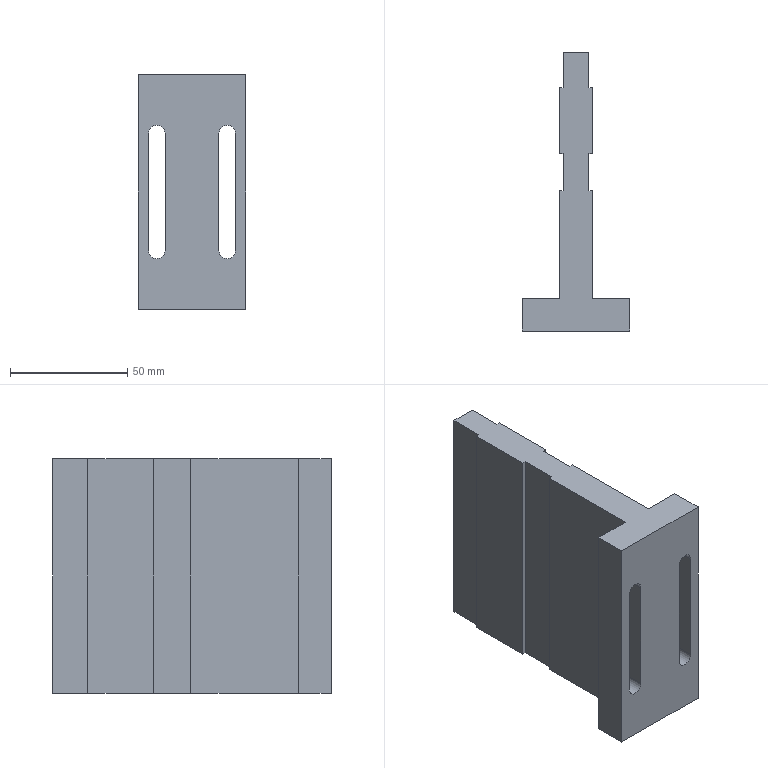Part | SolidWorks | features ICE 2, MirrorPattern 2, Extrusion 1 | 1 solid | 30 faces | box 46 x 119 x 100 mm | volume 191222 mm3 | plane 26 | cylinder 4 | commonest cylinder face diameters 7 x4
STEP:
#1=CARTESIAN_POINT('',(-5.5,119.,-50.));
#2=VERTEX_POINT('',#1);
#3=CARTESIAN_POINT('',(-5.5,119.,50.));
#4=VERTEX_POINT('',#3);
#5=CARTESIAN_POINT('',(-5.5,119.,50.));
#6=DIRECTION('',(0.,0.,1.));
#7=VECTOR('',#6,1000.);
#8=LINE('',#5,#7);
#9=EDGE_CURVE('',#2,#4,#8,.T.);
#10=ORIENTED_EDGE('',*,*,#9,.T.);
#11=CARTESIAN_POINT('',(5.5,119.,50.));
#12=VERTEX_POINT('',#11);
#13=CARTESIAN_POINT('',(7.,119.,50.));
#14=DIRECTION('',(-1.,0.,0.));
#15=VECTOR('',#14,1000.);
#16=LINE('',#13,#15);
#17=EDGE_CURVE('',#12,#4,#16,.T.);
#18=ORIENTED_EDGE('',*,*,#17,.F.);
#19=CARTESIAN_POINT('',(5.5,119.,-50.));
#20=VERTEX_POINT('',#19);
#21=CARTESIAN_POINT('',(5.5,119.,50.));
#22=DIRECTION('',(0.,0.,1.));
#23=VECTOR('',#22,1000.);
#24=LINE('',#21,#23);
#25=EDGE_CURVE('',#20,#12,#24,.T.);
#26=ORIENTED_EDGE('',*,*,#25,.F.);
#27=CARTESIAN_POINT('',(7.,119.,-50.));
#28=DIRECTION('',(-1.,0.,0.));
#29=VECTOR('',#28,1000.);
#30=LINE('',#27,#29);
#31=EDGE_CURVE('',#20,#2,#30,.T.);
#32=ORIENTED_EDGE('',*,*,#31,.T.);
#33=EDGE_LOOP('',(#10,#18,#26,#32));
#34=FACE_OUTER_BOUND('',#33,.T.);
#35=CARTESIAN_POINT('',(7.,119.,50.));
#36=DIRECTION('',(0.,-1.,0.));
#37=DIRECTION('',(0.,0.,-1.));
#38=AXIS2_PLACEMENT_3D('',#35,#36,#37);
#39=PLANE('',#38);
#40=ADVANCED_FACE('',(#34),#39,.F.);
#41=CARTESIAN_POINT('',(-7.,104.,50.));
#42=VERTEX_POINT('',#41);
#43=CARTESIAN_POINT('',(-7.,104.,-50.));
#44=VERTEX_POINT('',#43);
#45=CARTESIAN_POINT('',(-7.,104.,50.));
#46=DIRECTION('',(0.,0.,-1.));
#47=VECTOR('',#46,1000.);
#48=LINE('',#45,#47);
#49=EDGE_CURVE('',#42,#44,#48,.T.);
#50=ORIENTED_EDGE('',*,*,#49,.T.);
#51=CARTESIAN_POINT('',(-7.,76.,-50.));
#52=VERTEX_POINT('',#51);
#53=CARTESIAN_POINT('',(-7.,119.,-50.));
#54=DIRECTION('',(0.,-1.,0.));
#55=VECTOR('',#54,1000.);
#56=LINE('',#53,#55);
#57=EDGE_CURVE('',#44,#52,#56,.T.);
#58=ORIENTED_EDGE('',*,*,#57,.T.);
#59=CARTESIAN_POINT('',(-7.,76.,50.));
#60=VERTEX_POINT('',#59);
#61=CARTESIAN_POINT('',(-7.,76.,50.));
#62=DIRECTION('',(0.,0.,1.));
#63=VECTOR('',#62,1000.);
#64=LINE('',#61,#63);
#65=EDGE_CURVE('',#52,#60,#64,.T.);
#66=ORIENTED_EDGE('',*,*,#65,.T.);
#67=CARTESIAN_POINT('',(-7.,119.,50.));
#68=DIRECTION('',(0.,-1.,0.));
#69=VECTOR('',#68,1000.);
#70=LINE('',#67,#69);
#71=EDGE_CURVE('',#42,#60,#70,.T.);
#72=ORIENTED_EDGE('',*,*,#71,.F.);
#73=EDGE_LOOP('',(#50,#58,#66,#72));
#74=FACE_OUTER_BOUND('',#73,.T.);
#75=CARTESIAN_POINT('',(-7.,119.,50.));
#76=DIRECTION('',(1.,0.,0.));
#77=DIRECTION('',(0.,1.,0.));
#78=AXIS2_PLACEMENT_3D('',#75,#76,#77);
#79=PLANE('',#78);
#80=ADVANCED_FACE('',(#74),#79,.F.);
#81=CARTESIAN_POINT('',(-7.,60.,50.));
#82=VERTEX_POINT('',#81);
#83=CARTESIAN_POINT('',(-7.,60.,-50.));
#84=VERTEX_POINT('',#83);
#85=CARTESIAN_POINT('',(-7.,60.,50.));
#86=DIRECTION('',(0.,0.,-1.));
#87=VECTOR('',#86,1000.);
#88=LINE('',#85,#87);
#89=EDGE_CURVE('',#82,#84,#88,.T.);
#90=ORIENTED_EDGE('',*,*,#89,.T.);
#91=CARTESIAN_POINT('',(-7.,14.,-50.));
#92=VERTEX_POINT('',#91);
#93=CARTESIAN_POINT('',(-7.,119.,-50.));
#94=DIRECTION('',(0.,-1.,0.));
#95=VECTOR('',#94,1000.);
#96=LINE('',#93,#95);
#97=EDGE_CURVE('',#84,#92,#96,.T.);
#98=ORIENTED_EDGE('',*,*,#97,.T.);
#99=CARTESIAN_POINT('',(-7.,14.,50.));
#100=VERTEX_POINT('',#99);
#101=CARTESIAN_POINT('',(-7.,14.,50.));
#102=DIRECTION('',(0.,0.,-1.));
#103=VECTOR('',#102,1000.);
#104=LINE('',#101,#103);
#105=EDGE_CURVE('',#100,#92,#104,.T.);
#106=ORIENTED_EDGE('',*,*,#105,.F.);
#107=CARTESIAN_POINT('',(-7.,119.,50.));
#108=DIRECTION('',(0.,-1.,0.));
#109=VECTOR('',#108,1000.);
#110=LINE('',#107,#109);
#111=EDGE_CURVE('',#82,#100,#110,.T.);
#112=ORIENTED_EDGE('',*,*,#111,.F.);
#113=EDGE_LOOP('',(#90,#98,#106,#112));
#114=FACE_OUTER_BOUND('',#113,.T.);
#115=CARTESIAN_POINT('',(-7.,119.,50.));
#116=DIRECTION('',(1.,0.,0.));
#117=DIRECTION('',(0.,1.,0.));
#118=AXIS2_PLACEMENT_3D('',#115,#116,#117);
#119=PLANE('',#118);
#120=ADVANCED_FACE('',(#114),#119,.F.);
#121=CARTESIAN_POINT('',(-5.5,104.,50.));
#122=VERTEX_POINT('',#121);
#123=CARTESIAN_POINT('',(-5.5,119.,50.));
#124=DIRECTION('',(0.,-1.,0.));
#125=VECTOR('',#124,1000.);
#126=LINE('',#123,#125);
#127=EDGE_CURVE('',#4,#122,#126,.T.);
#128=ORIENTED_EDGE('',*,*,#127,.T.);
#129=CARTESIAN_POINT('',(-5.5,104.,50.));
#130=DIRECTION('',(-1.,0.,0.));
#131=VECTOR('',#130,1000.);
#132=LINE('',#129,#131);
#133=EDGE_CURVE('',#122,#42,#132,.T.);
#134=ORIENTED_EDGE('',*,*,#133,.T.);
#135=ORIENTED_EDGE('',*,*,#71,.T.);
#136=CARTESIAN_POINT('',(-5.5,76.,50.));
#137=VERTEX_POINT('',#136);
#138=CARTESIAN_POINT('',(-5.5,76.,50.));
#139=DIRECTION('',(-1.,0.,0.));
#140=VECTOR('',#139,1000.);
#141=LINE('',#138,#140);
#142=EDGE_CURVE('',#137,#60,#141,.T.);
#143=ORIENTED_EDGE('',*,*,#142,.F.);
#144=CARTESIAN_POINT('',(-5.5,60.,50.));
#145=VERTEX_POINT('',#144);
#146=CARTESIAN_POINT('',(-5.5,76.,50.));
#147=DIRECTION('',(0.,-1.,0.));
#148=VECTOR('',#147,1000.);
#149=LINE('',#146,#148);
#150=EDGE_CURVE('',#137,#145,#149,.T.);
#151=ORIENTED_EDGE('',*,*,#150,.T.);
#152=CARTESIAN_POINT('',(-5.5,60.,50.));
#153=DIRECTION('',(-1.,0.,0.));
#154=VECTOR('',#153,1000.);
#155=LINE('',#152,#154);
#156=EDGE_CURVE('',#145,#82,#155,.T.);
#157=ORIENTED_EDGE('',*,*,#156,.T.);
#158=ORIENTED_EDGE('',*,*,#111,.T.);
#159=CARTESIAN_POINT('',(-23.,14.,50.));
#160=VERTEX_POINT('',#159);
#161=CARTESIAN_POINT('',(-7.,14.,50.));
#162=DIRECTION('',(-1.,0.,0.));
#163=VECTOR('',#162,1000.);
#164=LINE('',#161,#163);
#165=EDGE_CURVE('',#100,#160,#164,.T.);
#166=ORIENTED_EDGE('',*,*,#165,.T.);
#167=CARTESIAN_POINT('',(-23.,0.,50.));
#168=VERTEX_POINT('',#167);
#169=CARTESIAN_POINT('',(-23.,14.,50.));
#170=DIRECTION('',(0.,-1.,0.));
#171=VECTOR('',#170,1000.);
#172=LINE('',#169,#171);
#173=EDGE_CURVE('',#160,#168,#172,.T.);
#174=ORIENTED_EDGE('',*,*,#173,.T.);
#175=CARTESIAN_POINT('',(23.,0.,50.));
#176=VERTEX_POINT('',#175);
#177=CARTESIAN_POINT('',(-23.,0.,50.));
#178=DIRECTION('',(1.,0.,0.));
#179=VECTOR('',#178,1000.);
#180=LINE('',#177,#179);
#181=EDGE_CURVE('',#168,#176,#180,.T.);
#182=ORIENTED_EDGE('',*,*,#181,.T.);
#183=CARTESIAN_POINT('',(23.,14.,50.));
#184=VERTEX_POINT('',#183);
#185=CARTESIAN_POINT('',(23.,0.,50.));
#186=DIRECTION('',(0.,1.,0.));
#187=VECTOR('',#186,1000.);
#188=LINE('',#185,#187);
#189=EDGE_CURVE('',#176,#184,#188,.T.);
#190=ORIENTED_EDGE('',*,*,#189,.T.);
#191=CARTESIAN_POINT('',(7.,14.,50.));
#192=VERTEX_POINT('',#191);
#193=CARTESIAN_POINT('',(23.,14.,50.));
#194=DIRECTION('',(-1.,0.,0.));
#195=VECTOR('',#194,1000.);
#196=LINE('',#193,#195);
#197=EDGE_CURVE('',#184,#192,#196,.T.);
#198=ORIENTED_EDGE('',*,*,#197,.T.);
#199=CARTESIAN_POINT('',(7.,60.,50.));
#200=VERTEX_POINT('',#199);
#201=CARTESIAN_POINT('',(7.,14.,50.));
#202=DIRECTION('',(0.,1.,0.));
#203=VECTOR('',#202,1000.);
#204=LINE('',#201,#203);
#205=EDGE_CURVE('',#192,#200,#204,.T.);
#206=ORIENTED_EDGE('',*,*,#205,.T.);
#207=CARTESIAN_POINT('',(5.5,60.,50.));
#208=VERTEX_POINT('',#207);
#209=CARTESIAN_POINT('',(5.5,60.,50.));
#210=DIRECTION('',(1.,0.,0.));
#211=VECTOR('',#210,1000.);
#212=LINE('',#209,#211);
#213=EDGE_CURVE('',#208,#200,#212,.T.);
#214=ORIENTED_EDGE('',*,*,#213,.F.);
#215=CARTESIAN_POINT('',(5.5,76.,50.));
#216=VERTEX_POINT('',#215);
#217=CARTESIAN_POINT('',(5.5,76.,50.));
#218=DIRECTION('',(0.,-1.,0.));
#219=VECTOR('',#218,1000.);
#220=LINE('',#217,#219);
#221=EDGE_CURVE('',#216,#208,#220,.T.);
#222=ORIENTED_EDGE('',*,*,#221,.F.);
#223=CARTESIAN_POINT('',(7.,76.,50.));
#224=VERTEX_POINT('',#223);
#225=CARTESIAN_POINT('',(5.5,76.,50.));
#226=DIRECTION('',(1.,0.,0.));
#227=VECTOR('',#226,1000.);
#228=LINE('',#225,#227);
#229=EDGE_CURVE('',#216,#224,#228,.T.);
#230=ORIENTED_EDGE('',*,*,#229,.T.);
#231=CARTESIAN_POINT('',(7.,104.,50.));
#232=VERTEX_POINT('',#231);
#233=CARTESIAN_POINT('',(7.,14.,50.));
#234=DIRECTION('',(0.,1.,0.));
#235=VECTOR('',#234,1000.);
#236=LINE('',#233,#235);
#237=EDGE_CURVE('',#224,#232,#236,.T.);
#238=ORIENTED_EDGE('',*,*,#237,.T.);
#239=CARTESIAN_POINT('',(5.5,104.,50.));
#240=VERTEX_POINT('',#239);
#241=CARTESIAN_POINT('',(5.5,104.,50.));
#242=DIRECTION('',(1.,0.,0.));
#243=VECTOR('',#242,1000.);
#244=LINE('',#241,#243);
#245=EDGE_CURVE('',#240,#232,#244,.T.);
#246=ORIENTED_EDGE('',*,*,#245,.F.);
#247=CARTESIAN_POINT('',(5.5,119.,50.));
#248=DIRECTION('',(0.,-1.,0.));
#249=VECTOR('',#248,1000.);
#250=LINE('',#247,#249);
#251=EDGE_CURVE('',#12,#240,#250,.T.);
#252=ORIENTED_EDGE('',*,*,#251,.F.);
#253=ORIENTED_EDGE('',*,*,#17,.T.);
#254=EDGE_LOOP('',(#128,#134,#135,#143,#151,#157,#158,#166,#174,#182,#190,#198,#206,#214,#222,#230,#238,#246,#252,#253));
#255=FACE_OUTER_BOUND('',#254,.T.);
#256=CARTESIAN_POINT('',(0.,0.,50.));
#257=DIRECTION('',(0.,0.,1.));
#258=DIRECTION('',(1.,0.,0.));
#259=AXIS2_PLACEMENT_3D('',#256,#257,#258);
#260=PLANE('',#259);
#261=ADVANCED_FACE('',(#255),#260,.T.);
#262=CARTESIAN_POINT('',(-5.5,104.,-50.));
#263=VERTEX_POINT('',#262);
#264=CARTESIAN_POINT('',(-5.5,104.,-50.));
#265=DIRECTION('',(-1.,0.,0.));
#266=VECTOR('',#265,1000.);
#267=LINE('',#264,#266);
#268=EDGE_CURVE('',#263,#44,#267,.T.);
#269=ORIENTED_EDGE('',*,*,#268,.F.);
#270=CARTESIAN_POINT('',(-5.5,119.,-50.));
#271=DIRECTION('',(0.,1.,0.));
#272=VECTOR('',#271,1000.);
#273=LINE('',#270,#272);
#274=EDGE_CURVE('',#263,#2,#273,.T.);
#275=ORIENTED_EDGE('',*,*,#274,.T.);
#276=ORIENTED_EDGE('',*,*,#31,.F.);
#277=CARTESIAN_POINT('',(5.5,104.,-50.));
#278=VERTEX_POINT('',#277);
#279=CARTESIAN_POINT('',(5.5,119.,-50.));
#280=DIRECTION('',(0.,1.,0.));
#281=VECTOR('',#280,1000.);
#282=LINE('',#279,#281);
#283=EDGE_CURVE('',#278,#20,#282,.T.);
#284=ORIENTED_EDGE('',*,*,#283,.F.);
#285=CARTESIAN_POINT('',(7.,104.,-50.));
#286=VERTEX_POINT('',#285);
#287=CARTESIAN_POINT('',(5.5,104.,-50.));
#288=DIRECTION('',(1.,0.,0.));
#289=VECTOR('',#288,1000.);
#290=LINE('',#287,#289);
#291=EDGE_CURVE('',#278,#286,#290,.T.);
#292=ORIENTED_EDGE('',*,*,#291,.T.);
#293=CARTESIAN_POINT('',(7.,76.,-50.));
#294=VERTEX_POINT('',#293);
#295=CARTESIAN_POINT('',(7.,14.,-50.));
#296=DIRECTION('',(0.,1.,0.));
#297=VECTOR('',#296,1000.);
#298=LINE('',#295,#297);
#299=EDGE_CURVE('',#294,#286,#298,.T.);
#300=ORIENTED_EDGE('',*,*,#299,.F.);
#301=CARTESIAN_POINT('',(5.5,76.,-50.));
#302=VERTEX_POINT('',#301);
#303=CARTESIAN_POINT('',(5.5,76.,-50.));
#304=DIRECTION('',(1.,0.,0.));
#305=VECTOR('',#304,1000.);
#306=LINE('',#303,#305);
#307=EDGE_CURVE('',#302,#294,#306,.T.);
#308=ORIENTED_EDGE('',*,*,#307,.F.);
#309=CARTESIAN_POINT('',(5.5,60.,-50.));
#310=VERTEX_POINT('',#309);
#311=CARTESIAN_POINT('',(5.5,76.,-50.));
#312=DIRECTION('',(0.,1.,0.));
#313=VECTOR('',#312,1000.);
#314=LINE('',#311,#313);
#315=EDGE_CURVE('',#310,#302,#314,.T.);
#316=ORIENTED_EDGE('',*,*,#315,.F.);
#317=CARTESIAN_POINT('',(7.,60.,-50.));
#318=VERTEX_POINT('',#317);
#319=CARTESIAN_POINT('',(5.5,60.,-50.));
#320=DIRECTION('',(1.,0.,0.));
#321=VECTOR('',#320,1000.);
#322=LINE('',#319,#321);
#323=EDGE_CURVE('',#310,#318,#322,.T.);
#324=ORIENTED_EDGE('',*,*,#323,.T.);
#325=CARTESIAN_POINT('',(7.,14.,-50.));
#326=VERTEX_POINT('',#325);
#327=CARTESIAN_POINT('',(7.,14.,-50.));
#328=DIRECTION('',(0.,1.,0.));
#329=VECTOR('',#328,1000.);
#330=LINE('',#327,#329);
#331=EDGE_CURVE('',#326,#318,#330,.T.);
#332=ORIENTED_EDGE('',*,*,#331,.F.);
#333=CARTESIAN_POINT('',(23.,14.,-50.));
#334=VERTEX_POINT('',#333);
#335=CARTESIAN_POINT('',(23.,14.,-50.));
#336=DIRECTION('',(-1.,0.,0.));
#337=VECTOR('',#336,1000.);
#338=LINE('',#335,#337);
#339=EDGE_CURVE('',#334,#326,#338,.T.);
#340=ORIENTED_EDGE('',*,*,#339,.F.);
#341=CARTESIAN_POINT('',(23.,0.,-50.));
#342=VERTEX_POINT('',#341);
#343=CARTESIAN_POINT('',(23.,0.,-50.));
#344=DIRECTION('',(0.,1.,0.));
#345=VECTOR('',#344,1000.);
#346=LINE('',#343,#345);
#347=EDGE_CURVE('',#342,#334,#346,.T.);
#348=ORIENTED_EDGE('',*,*,#347,.F.);
#349=CARTESIAN_POINT('',(-23.,0.,-50.));
#350=VERTEX_POINT('',#349);
#351=CARTESIAN_POINT('',(0.,0.,-50.));
#352=DIRECTION('',(1.,0.,0.));
#353=VECTOR('',#352,1000.);
#354=LINE('',#351,#353);
#355=EDGE_CURVE('',#350,#342,#354,.T.);
#356=ORIENTED_EDGE('',*,*,#355,.F.);
#357=CARTESIAN_POINT('',(-23.,14.,-50.));
#358=VERTEX_POINT('',#357);
#359=CARTESIAN_POINT('',(-23.,14.,-50.));
#360=DIRECTION('',(0.,-1.,0.));
#361=VECTOR('',#360,1000.);
#362=LINE('',#359,#361);
#363=EDGE_CURVE('',#358,#350,#362,.T.);
#364=ORIENTED_EDGE('',*,*,#363,.F.);
#365=CARTESIAN_POINT('',(-7.,14.,-50.));
#366=DIRECTION('',(-1.,0.,0.));
#367=VECTOR('',#366,1000.);
#368=LINE('',#365,#367);
#369=EDGE_CURVE('',#92,#358,#368,.T.);
#370=ORIENTED_EDGE('',*,*,#369,.F.);
#371=ORIENTED_EDGE('',*,*,#97,.F.);
#372=CARTESIAN_POINT('',(-5.5,60.,-50.));
#373=VERTEX_POINT('',#372);
#374=CARTESIAN_POINT('',(-5.5,60.,-50.));
#375=DIRECTION('',(-1.,0.,0.));
#376=VECTOR('',#375,1000.);
#377=LINE('',#374,#376);
#378=EDGE_CURVE('',#373,#84,#377,.T.);
#379=ORIENTED_EDGE('',*,*,#378,.F.);
#380=CARTESIAN_POINT('',(-5.5,76.,-50.));
#381=VERTEX_POINT('',#380);
#382=CARTESIAN_POINT('',(-5.5,76.,-50.));
#383=DIRECTION('',(0.,1.,0.));
#384=VECTOR('',#383,1000.);
#385=LINE('',#382,#384);
#386=EDGE_CURVE('',#373,#381,#385,.T.);
#387=ORIENTED_EDGE('',*,*,#386,.T.);
#388=CARTESIAN_POINT('',(-5.5,76.,-50.));
#389=DIRECTION('',(-1.,0.,0.));
#390=VECTOR('',#389,1000.);
#391=LINE('',#388,#390);
#392=EDGE_CURVE('',#381,#52,#391,.T.);
#393=ORIENTED_EDGE('',*,*,#392,.T.);
#394=ORIENTED_EDGE('',*,*,#57,.F.);
#395=EDGE_LOOP('',(#269,#275,#276,#284,#292,#300,#308,#316,#324,#332,#340,#348,#356,#364,#370,#371,#379,#387,#393,#394));
#396=FACE_OUTER_BOUND('',#395,.T.);
#397=CARTESIAN_POINT('',(0.,0.,-50.));
#398=DIRECTION('',(0.,0.,1.));
#399=DIRECTION('',(1.,0.,0.));
#400=AXIS2_PLACEMENT_3D('',#397,#398,#399);
#401=PLANE('',#400);
#402=ADVANCED_FACE('',(#396),#401,.F.);
#403=ORIENTED_EDGE('',*,*,#355,.T.);
#404=CARTESIAN_POINT('',(23.,0.,50.));
#405=DIRECTION('',(0.,0.,-1.));
#406=VECTOR('',#405,1000.);
#407=LINE('',#404,#406);
#408=EDGE_CURVE('',#176,#342,#407,.T.);
#409=ORIENTED_EDGE('',*,*,#408,.F.);
#410=ORIENTED_EDGE('',*,*,#181,.F.);
#411=CARTESIAN_POINT('',(-23.,0.,50.));
#412=DIRECTION('',(0.,0.,-1.));
#413=VECTOR('',#412,1000.);
#414=LINE('',#411,#413);
#415=EDGE_CURVE('',#168,#350,#414,.T.);
#416=ORIENTED_EDGE('',*,*,#415,.T.);
#417=EDGE_LOOP('',(#403,#409,#410,#416));
#418=FACE_OUTER_BOUND('',#417,.T.);
#419=CARTESIAN_POINT('',(11.5,0.,25.));
#420=VERTEX_POINT('',#419);
#421=CARTESIAN_POINT('',(11.5,0.,-25.));
#422=VERTEX_POINT('',#421);
#423=CARTESIAN_POINT('',(11.5,0.,25.));
#424=DIRECTION('',(0.,0.,-1.));
#425=VECTOR('',#424,1000.);
#426=LINE('',#423,#425);
#427=EDGE_CURVE('',#420,#422,#426,.T.);
#428=ORIENTED_EDGE('',*,*,#427,.F.);
#429=CARTESIAN_POINT('',(18.5,0.,25.));
#430=VERTEX_POINT('',#429);
#431=CARTESIAN_POINT('',(15.,0.,25.));
#432=DIRECTION('',(0.,-1.,0.));
#433=DIRECTION('',(0.,0.,1.));
#434=AXIS2_PLACEMENT_3D('',#431,#432,#433);
#435=CIRCLE('',#434,3.5);
#436=EDGE_CURVE('',#430,#420,#435,.T.);
#437=ORIENTED_EDGE('',*,*,#436,.F.);
#438=CARTESIAN_POINT('',(18.5,0.,-25.));
#439=VERTEX_POINT('',#438);
#440=CARTESIAN_POINT('',(18.5,0.,25.));
#441=DIRECTION('',(0.,0.,1.));
#442=VECTOR('',#441,1000.);
#443=LINE('',#440,#442);
#444=EDGE_CURVE('',#439,#430,#443,.T.);
#445=ORIENTED_EDGE('',*,*,#444,.F.);
#446=CARTESIAN_POINT('',(15.,0.,-25.));
#447=DIRECTION('',(0.,-1.,0.));
#448=DIRECTION('',(0.,0.,1.));
#449=AXIS2_PLACEMENT_3D('',#446,#447,#448);
#450=CIRCLE('',#449,3.5);
#451=EDGE_CURVE('',#422,#439,#450,.T.);
#452=ORIENTED_EDGE('',*,*,#451,.F.);
#453=EDGE_LOOP('',(#428,#437,#445,#452));
#454=FACE_BOUND('',#453,.T.);
#455=CARTESIAN_POINT('',(-18.5,0.,25.));
#456=VERTEX_POINT('',#455);
#457=CARTESIAN_POINT('',(-11.5,0.,25.));
#458=VERTEX_POINT('',#457);
#459=CARTESIAN_POINT('',(-15.,0.,25.));
#460=DIRECTION('',(0.,1.,0.));
#461=DIRECTION('',(0.,0.,1.));
#462=AXIS2_PLACEMENT_3D('',#459,#460,#461);
#463=CIRCLE('',#462,3.5);
#464=EDGE_CURVE('',#456,#458,#463,.T.);
#465=ORIENTED_EDGE('',*,*,#464,.T.);
#466=CARTESIAN_POINT('',(-11.5,0.,-25.));
#467=VERTEX_POINT('',#466);
#468=CARTESIAN_POINT('',(-11.5,0.,25.));
#469=DIRECTION('',(0.,0.,-1.));
#470=VECTOR('',#469,1000.);
#471=LINE('',#468,#470);
#472=EDGE_CURVE('',#458,#467,#471,.T.);
#473=ORIENTED_EDGE('',*,*,#472,.T.);
#474=CARTESIAN_POINT('',(-18.5,0.,-25.));
#475=VERTEX_POINT('',#474);
#476=CARTESIAN_POINT('',(-15.,0.,-25.));
#477=DIRECTION('',(0.,1.,0.));
#478=DIRECTION('',(0.,0.,1.));
#479=AXIS2_PLACEMENT_3D('',#476,#477,#478);
#480=CIRCLE('',#479,3.5);
#481=EDGE_CURVE('',#467,#475,#480,.T.);
#482=ORIENTED_EDGE('',*,*,#481,.T.);
#483=CARTESIAN_POINT('',(-18.5,0.,25.));
#484=DIRECTION('',(0.,0.,1.));
#485=VECTOR('',#484,1000.);
#486=LINE('',#483,#485);
#487=EDGE_CURVE('',#475,#456,#486,.T.);
#488=ORIENTED_EDGE('',*,*,#487,.T.);
#489=EDGE_LOOP('',(#465,#473,#482,#488));
#490=FACE_BOUND('',#489,.T.);
#491=CARTESIAN_POINT('',(0.,0.,50.));
#492=DIRECTION('',(0.,1.,0.));
#493=DIRECTION('',(0.,0.,1.));
#494=AXIS2_PLACEMENT_3D('',#491,#492,#493);
#495=PLANE('',#494);
#496=ADVANCED_FACE('',(#418,#454,#490),#495,.F.);
#497=ORIENTED_EDGE('',*,*,#369,.T.);
#498=CARTESIAN_POINT('',(-23.,14.,50.));
#499=DIRECTION('',(0.,0.,-1.));
#500=VECTOR('',#499,1000.);
#501=LINE('',#498,#500);
#502=EDGE_CURVE('',#160,#358,#501,.T.);
#503=ORIENTED_EDGE('',*,*,#502,.F.);
#504=ORIENTED_EDGE('',*,*,#165,.F.);
#505=ORIENTED_EDGE('',*,*,#105,.T.);
#506=EDGE_LOOP('',(#497,#503,#504,#505));
#507=FACE_OUTER_BOUND('',#506,.T.);
#508=CARTESIAN_POINT('',(-11.5,14.,25.));
#509=VERTEX_POINT('',#508);
#510=CARTESIAN_POINT('',(-18.5,14.,25.));
#511=VERTEX_POINT('',#510);
#512=CARTESIAN_POINT('',(-15.,14.,25.));
#513=DIRECTION('',(0.,-1.,0.));
#514=DIRECTION('',(1.,0.,0.));
#515=AXIS2_PLACEMENT_3D('',#512,#513,#514);
#516=CIRCLE('',#515,3.5);
#517=EDGE_CURVE('',#509,#511,#516,.T.);
#518=ORIENTED_EDGE('',*,*,#517,.T.);
#519=CARTESIAN_POINT('',(-18.5,14.,-25.));
#520=VERTEX_POINT('',#519);
#521=CARTESIAN_POINT('',(-18.5,14.,25.));
#522=DIRECTION('',(0.,0.,-1.));
#523=VECTOR('',#522,1000.);
#524=LINE('',#521,#523);
#525=EDGE_CURVE('',#511,#520,#524,.T.);
#526=ORIENTED_EDGE('',*,*,#525,.T.);
#527=CARTESIAN_POINT('',(-11.5,14.,-25.));
#528=VERTEX_POINT('',#527);
#529=CARTESIAN_POINT('',(-15.,14.,-25.));
#530=DIRECTION('',(0.,-1.,0.));
#531=DIRECTION('',(1.,0.,0.));
#532=AXIS2_PLACEMENT_3D('',#529,#530,#531);
#533=CIRCLE('',#532,3.5);
#534=EDGE_CURVE('',#520,#528,#533,.T.);
#535=ORIENTED_EDGE('',*,*,#534,.T.);
#536=CARTESIAN_POINT('',(-11.5,14.,25.));
#537=DIRECTION('',(0.,0.,1.));
#538=VECTOR('',#537,1000.);
#539=LINE('',#536,#538);
#540=EDGE_CURVE('',#528,#509,#539,.T.);
#541=ORIENTED_EDGE('',*,*,#540,.T.);
#542=EDGE_LOOP('',(#518,#526,#535,#541));
#543=FACE_BOUND('',#542,.T.);
#544=CARTESIAN_POINT('',(-7.,14.,50.));
#545=DIRECTION('',(0.,-1.,0.));
#546=DIRECTION('',(0.,0.,-1.));
#547=AXIS2_PLACEMENT_3D('',#544,#545,#546);
#548=PLANE('',#547);
#549=ADVANCED_FACE('',(#507,#543),#548,.F.);
#550=ORIENTED_EDGE('',*,*,#299,.T.);
#551=CARTESIAN_POINT('',(7.,104.,50.));
#552=DIRECTION('',(0.,0.,-1.));
#553=VECTOR('',#552,1000.);
#554=LINE('',#551,#553);
#555=EDGE_CURVE('',#232,#286,#554,.T.);
#556=ORIENTED_EDGE('',*,*,#555,.F.);
#557=ORIENTED_EDGE('',*,*,#237,.F.);
#558=CARTESIAN_POINT('',(7.,76.,50.));
#559=DIRECTION('',(0.,0.,1.));
#560=VECTOR('',#559,1000.);
#561=LINE('',#558,#560);
#562=EDGE_CURVE('',#294,#224,#561,.T.);
#563=ORIENTED_EDGE('',*,*,#562,.F.);
#564=EDGE_LOOP('',(#550,#556,#557,#563));
#565=FACE_OUTER_BOUND('',#564,.T.);
#566=CARTESIAN_POINT('',(7.,14.,50.));
#567=DIRECTION('',(-1.,0.,0.));
#568=DIRECTION('',(0.,-1.,0.));
#569=AXIS2_PLACEMENT_3D('',#566,#567,#568);
#570=PLANE('',#569);
#571=ADVANCED_FACE('',(#565),#570,.F.);
#572=ORIENTED_EDGE('',*,*,#347,.T.);
#573=CARTESIAN_POINT('',(23.,14.,50.));
#574=DIRECTION('',(0.,0.,-1.));
#575=VECTOR('',#574,1000.);
#576=LINE('',#573,#575);
#577=EDGE_CURVE('',#184,#334,#576,.T.);
#578=ORIENTED_EDGE('',*,*,#577,.F.);
#579=ORIENTED_EDGE('',*,*,#189,.F.);
#580=ORIENTED_EDGE('',*,*,#408,.T.);
#581=EDGE_LOOP('',(#572,#578,#579,#580));
#582=FACE_OUTER_BOUND('',#581,.T.);
#583=CARTESIAN_POINT('',(23.,0.,50.));
#584=DIRECTION('',(-1.,0.,0.));
#585=DIRECTION('',(0.,0.,1.));
#586=AXIS2_PLACEMENT_3D('',#583,#584,#585);
#587=PLANE('',#586);
#588=ADVANCED_FACE('',(#582),#587,.F.);
#589=CARTESIAN_POINT('',(18.5,14.,25.));
#590=VERTEX_POINT('',#589);
#591=CARTESIAN_POINT('',(18.5,14.,-25.));
#592=VERTEX_POINT('',#591);
#593=CARTESIAN_POINT('',(18.5,14.,25.));
#594=DIRECTION('',(0.,0.,-1.));
#595=VECTOR('',#594,1000.);
#596=LINE('',#593,#595);
#597=EDGE_CURVE('',#590,#592,#596,.T.);
#598=ORIENTED_EDGE('',*,*,#597,.F.);
#599=CARTESIAN_POINT('',(11.5,14.,25.));
#600=VERTEX_POINT('',#599);
#601=CARTESIAN_POINT('',(15.,14.,25.));
#602=DIRECTION('',(0.,1.,0.));
#603=DIRECTION('',(-1.,0.,0.));
#604=AXIS2_PLACEMENT_3D('',#601,#602,#603);
#605=CIRCLE('',#604,3.5);
#606=EDGE_CURVE('',#600,#590,#605,.T.);
#607=ORIENTED_EDGE('',*,*,#606,.F.);
#608=CARTESIAN_POINT('',(11.5,14.,-25.));
#609=VERTEX_POINT('',#608);
#610=CARTESIAN_POINT('',(11.5,14.,25.));
#611=DIRECTION('',(0.,0.,1.));
#612=VECTOR('',#611,1000.);
#613=LINE('',#610,#612);
#614=EDGE_CURVE('',#609,#600,#613,.T.);
#615=ORIENTED_EDGE('',*,*,#614,.F.);
#616=CARTESIAN_POINT('',(15.,14.,-25.));
#617=DIRECTION('',(0.,1.,0.));
#618=DIRECTION('',(-1.,0.,0.));
#619=AXIS2_PLACEMENT_3D('',#616,#617,#618);
#620=CIRCLE('',#619,3.5);
#621=EDGE_CURVE('',#592,#609,#620,.T.);
#622=ORIENTED_EDGE('',*,*,#621,.F.);
#623=EDGE_LOOP('',(#598,#607,#615,#622));
#624=FACE_BOUND('',#623,.T.);
#625=ORIENTED_EDGE('',*,*,#339,.T.);
#626=CARTESIAN_POINT('',(7.,14.,50.));
#627=DIRECTION('',(0.,0.,-1.));
#628=VECTOR('',#627,1000.);
#629=LINE('',#626,#628);
#630=EDGE_CURVE('',#192,#326,#629,.T.);
#631=ORIENTED_EDGE('',*,*,#630,.F.);
#632=ORIENTED_EDGE('',*,*,#197,.F.);
#633=ORIENTED_EDGE('',*,*,#577,.T.);
#634=EDGE_LOOP('',(#625,#631,#632,#633));
#635=FACE_OUTER_BOUND('',#634,.T.);
#636=CARTESIAN_POINT('',(23.,14.,50.));
#637=DIRECTION('',(0.,-1.,0.));
#638=DIRECTION('',(0.,0.,-1.));
#639=AXIS2_PLACEMENT_3D('',#636,#637,#638);
#640=PLANE('',#639);
#641=ADVANCED_FACE('',(#624,#635),#640,.F.);
#642=ORIENTED_EDGE('',*,*,#331,.T.);
#643=CARTESIAN_POINT('',(7.,60.,50.));
#644=DIRECTION('',(0.,0.,-1.));
#645=VECTOR('',#644,1000.);
#646=LINE('',#643,#645);
#647=EDGE_CURVE('',#200,#318,#646,.T.);
#648=ORIENTED_EDGE('',*,*,#647,.F.);
#649=ORIENTED_EDGE('',*,*,#205,.F.);
#650=ORIENTED_EDGE('',*,*,#630,.T.);
#651=EDGE_LOOP('',(#642,#648,#649,#650));
#652=FACE_OUTER_BOUND('',#651,.T.);
#653=CARTESIAN_POINT('',(7.,14.,50.));
#654=DIRECTION('',(-1.,0.,0.));
#655=DIRECTION('',(0.,-1.,0.));
#656=AXIS2_PLACEMENT_3D('',#653,#654,#655);
#657=PLANE('',#656);
#658=ADVANCED_FACE('',(#652),#657,.F.);
#659=ORIENTED_EDGE('',*,*,#363,.T.);
#660=ORIENTED_EDGE('',*,*,#415,.F.);
#661=ORIENTED_EDGE('',*,*,#173,.F.);
#662=ORIENTED_EDGE('',*,*,#502,.T.);
#663=EDGE_LOOP('',(#659,#660,#661,#662));
#664=FACE_OUTER_BOUND('',#663,.T.);
#665=CARTESIAN_POINT('',(-23.,14.,50.));
#666=DIRECTION('',(1.,0.,0.));
#667=DIRECTION('',(0.,1.,0.));
#668=AXIS2_PLACEMENT_3D('',#665,#666,#667);
#669=PLANE('',#668);
#670=ADVANCED_FACE('',(#664),#669,.F.);
#671=ORIENTED_EDGE('',*,*,#436,.T.);
#672=CARTESIAN_POINT('',(11.5,-0.001,25.));
#673=DIRECTION('',(0.,1.,0.));
#674=VECTOR('',#673,1000.);
#675=LINE('',#672,#674);
#676=EDGE_CURVE('',#420,#600,#675,.T.);
#677=ORIENTED_EDGE('',*,*,#676,.T.);
#678=ORIENTED_EDGE('',*,*,#606,.T.);
#679=CARTESIAN_POINT('',(18.5,-0.001,25.));
#680=DIRECTION('',(0.,1.,0.));
#681=VECTOR('',#680,1000.);
#682=LINE('',#679,#681);
#683=EDGE_CURVE('',#430,#590,#682,.T.);
#684=ORIENTED_EDGE('',*,*,#683,.F.);
#685=EDGE_LOOP('',(#671,#677,#678,#684));
#686=FACE_OUTER_BOUND('',#685,.T.);
#687=CARTESIAN_POINT('',(15.,-0.001,25.));
#688=DIRECTION('',(0.,1.,0.));
#689=DIRECTION('',(-1.,0.,0.));
#690=AXIS2_PLACEMENT_3D('',#687,#688,#689);
#691=CYLINDRICAL_SURFACE('',#690,3.5);
#692=ADVANCED_FACE('',(#686),#691,.F.);
#693=ORIENTED_EDGE('',*,*,#427,.T.);
#694=CARTESIAN_POINT('',(11.5,-0.001,-25.));
#695=DIRECTION('',(0.,1.,0.));
#696=VECTOR('',#695,1000.);
#697=LINE('',#694,#696);
#698=EDGE_CURVE('',#422,#609,#697,.T.);
#699=ORIENTED_EDGE('',*,*,#698,.T.);
#700=ORIENTED_EDGE('',*,*,#614,.T.);
#701=ORIENTED_EDGE('',*,*,#676,.F.);
#702=EDGE_LOOP('',(#693,#699,#700,#701));
#703=FACE_OUTER_BOUND('',#702,.T.);
#704=CARTESIAN_POINT('',(11.5,-0.001,25.));
#705=DIRECTION('',(-1.,0.,0.));
#706=DIRECTION('',(0.,-1.,0.));
#707=AXIS2_PLACEMENT_3D('',#704,#705,#706);
#708=PLANE('',#707);
#709=ADVANCED_FACE('',(#703),#708,.F.);
#710=ORIENTED_EDGE('',*,*,#451,.T.);
#711=CARTESIAN_POINT('',(18.5,-0.001,-25.));
#712=DIRECTION('',(0.,1.,0.));
#713=VECTOR('',#712,1000.);
#714=LINE('',#711,#713);
#715=EDGE_CURVE('',#439,#592,#714,.T.);
#716=ORIENTED_EDGE('',*,*,#715,.T.);
#717=ORIENTED_EDGE('',*,*,#621,.T.);
#718=ORIENTED_EDGE('',*,*,#698,.F.);
#719=EDGE_LOOP('',(#710,#716,#717,#718));
#720=FACE_OUTER_BOUND('',#719,.T.);
#721=CARTESIAN_POINT('',(15.,-0.001,-25.));
#722=DIRECTION('',(0.,1.,0.));
#723=DIRECTION('',(-1.,0.,0.));
#724=AXIS2_PLACEMENT_3D('',#721,#722,#723);
#725=CYLINDRICAL_SURFACE('',#724,3.5);
#726=ADVANCED_FACE('',(#720),#725,.F.);
#727=ORIENTED_EDGE('',*,*,#444,.T.);
#728=ORIENTED_EDGE('',*,*,#683,.T.);
#729=ORIENTED_EDGE('',*,*,#597,.T.);
#730=ORIENTED_EDGE('',*,*,#715,.F.);
#731=EDGE_LOOP('',(#727,#728,#729,#730));
#732=FACE_OUTER_BOUND('',#731,.T.);
#733=CARTESIAN_POINT('',(18.5,-0.001,25.));
#734=DIRECTION('',(1.,0.,0.));
#735=DIRECTION('',(0.,1.,0.));
#736=AXIS2_PLACEMENT_3D('',#733,#734,#735);
#737=PLANE('',#736);
#738=ADVANCED_FACE('',(#732),#737,.F.);
#739=ORIENTED_EDGE('',*,*,#562,.T.);
#740=ORIENTED_EDGE('',*,*,#229,.F.);
#741=CARTESIAN_POINT('',(5.5,76.,50.));
#742=DIRECTION('',(0.,0.,1.));
#743=VECTOR('',#742,1000.);
#744=LINE('',#741,#743);
#745=EDGE_CURVE('',#302,#216,#744,.T.);
#746=ORIENTED_EDGE('',*,*,#745,.F.);
#747=ORIENTED_EDGE('',*,*,#307,.T.);
#748=EDGE_LOOP('',(#739,#740,#746,#747));
#749=FACE_OUTER_BOUND('',#748,.T.);
#750=CARTESIAN_POINT('',(5.5,76.,50.));
#751=DIRECTION('',(0.,1.,0.));
#752=DIRECTION('',(-1.,0.,0.));
#753=AXIS2_PLACEMENT_3D('',#750,#751,#752);
#754=PLANE('',#753);
#755=ADVANCED_FACE('',(#749),#754,.F.);
#756=ORIENTED_EDGE('',*,*,#647,.T.);
#757=ORIENTED_EDGE('',*,*,#323,.F.);
#758=CARTESIAN_POINT('',(5.5,60.,50.));
#759=DIRECTION('',(0.,0.,-1.));
#760=VECTOR('',#759,1000.);
#761=LINE('',#758,#760);
#762=EDGE_CURVE('',#208,#310,#761,.T.);
#763=ORIENTED_EDGE('',*,*,#762,.F.);
#764=ORIENTED_EDGE('',*,*,#213,.T.);
#765=EDGE_LOOP('',(#756,#757,#763,#764));
#766=FACE_OUTER_BOUND('',#765,.T.);
#767=CARTESIAN_POINT('',(5.5,60.,50.));
#768=DIRECTION('',(0.,-1.,0.));
#769=DIRECTION('',(1.,0.,0.));
#770=AXIS2_PLACEMENT_3D('',#767,#768,#769);
#771=PLANE('',#770);
#772=ADVANCED_FACE('',(#766),#771,.F.);
#773=ORIENTED_EDGE('',*,*,#221,.T.);
#774=ORIENTED_EDGE('',*,*,#762,.T.);
#775=ORIENTED_EDGE('',*,*,#315,.T.);
#776=ORIENTED_EDGE('',*,*,#745,.T.);
#777=EDGE_LOOP('',(#773,#774,#775,#776));
#778=FACE_OUTER_BOUND('',#777,.T.);
#779=CARTESIAN_POINT('',(5.5,0.,0.));
#780=DIRECTION('',(1.,0.,0.));
#781=DIRECTION('',(0.,1.,0.));
#782=AXIS2_PLACEMENT_3D('',#779,#780,#781);
#783=PLANE('',#782);
#784=ADVANCED_FACE('',(#778),#783,.T.);
#785=ORIENTED_EDGE('',*,*,#555,.T.);
#786=ORIENTED_EDGE('',*,*,#291,.F.);
#787=CARTESIAN_POINT('',(5.5,104.,50.));
#788=DIRECTION('',(0.,0.,-1.));
#789=VECTOR('',#788,1000.);
#790=LINE('',#787,#789);
#791=EDGE_CURVE('',#240,#278,#790,.T.);
#792=ORIENTED_EDGE('',*,*,#791,.F.);
#793=ORIENTED_EDGE('',*,*,#245,.T.);
#794=EDGE_LOOP('',(#785,#786,#792,#793));
#795=FACE_OUTER_BOUND('',#794,.T.);
#796=CARTESIAN_POINT('',(5.5,104.,50.));
#797=DIRECTION('',(0.,-1.,0.));
#798=DIRECTION('',(1.,0.,0.));
#799=AXIS2_PLACEMENT_3D('',#796,#797,#798);
#800=PLANE('',#799);
#801=ADVANCED_FACE('',(#795),#800,.F.);
#802=ORIENTED_EDGE('',*,*,#251,.T.);
#803=ORIENTED_EDGE('',*,*,#791,.T.);
#804=ORIENTED_EDGE('',*,*,#283,.T.);
#805=ORIENTED_EDGE('',*,*,#25,.T.);
#806=EDGE_LOOP('',(#802,#803,#804,#805));
#807=FACE_OUTER_BOUND('',#806,.T.);
#808=CARTESIAN_POINT('',(5.5,0.,0.));
#809=DIRECTION('',(1.,0.,0.));
#810=DIRECTION('',(0.,1.,0.));
#811=AXIS2_PLACEMENT_3D('',#808,#809,#810);
#812=PLANE('',#811);
#813=ADVANCED_FACE('',(#807),#812,.T.);
#814=CARTESIAN_POINT('',(-18.5,-0.001,25.));
#815=DIRECTION('',(0.,1.,0.));
#816=VECTOR('',#815,1000.);
#817=LINE('',#814,#816);
#818=EDGE_CURVE('',#456,#511,#817,.T.);
#819=ORIENTED_EDGE('',*,*,#818,.T.);
#820=ORIENTED_EDGE('',*,*,#517,.F.);
#821=CARTESIAN_POINT('',(-11.5,-0.001,25.));
#822=DIRECTION('',(0.,1.,0.));
#823=VECTOR('',#822,1000.);
#824=LINE('',#821,#823);
#825=EDGE_CURVE('',#458,#509,#824,.T.);
#826=ORIENTED_EDGE('',*,*,#825,.F.);
#827=ORIENTED_EDGE('',*,*,#464,.F.);
#828=EDGE_LOOP('',(#819,#820,#826,#827));
#829=FACE_OUTER_BOUND('',#828,.T.);
#830=CARTESIAN_POINT('',(-15.,-0.001,25.));
#831=DIRECTION('',(0.,1.,0.));
#832=DIRECTION('',(-1.,0.,0.));
#833=AXIS2_PLACEMENT_3D('',#830,#831,#832);
#834=CYLINDRICAL_SURFACE('',#833,3.5);
#835=ADVANCED_FACE('',(#829),#834,.F.);
#836=CARTESIAN_POINT('',(-18.5,-0.001,-25.));
#837=DIRECTION('',(0.,1.,0.));
#838=VECTOR('',#837,1000.);
#839=LINE('',#836,#838);
#840=EDGE_CURVE('',#475,#520,#839,.T.);
#841=ORIENTED_EDGE('',*,*,#840,.T.);
#842=ORIENTED_EDGE('',*,*,#525,.F.);
#843=ORIENTED_EDGE('',*,*,#818,.F.);
#844=ORIENTED_EDGE('',*,*,#487,.F.);
#845=EDGE_LOOP('',(#841,#842,#843,#844));
#846=FACE_OUTER_BOUND('',#845,.T.);
#847=CARTESIAN_POINT('',(-18.5,-0.001,25.));
#848=DIRECTION('',(1.,0.,0.));
#849=DIRECTION('',(0.,1.,0.));
#850=AXIS2_PLACEMENT_3D('',#847,#848,#849);
#851=PLANE('',#850);
#852=ADVANCED_FACE('',(#846),#851,.T.);
#853=CARTESIAN_POINT('',(-11.5,-0.001,-25.));
#854=DIRECTION('',(0.,1.,0.));
#855=VECTOR('',#854,1000.);
#856=LINE('',#853,#855);
#857=EDGE_CURVE('',#467,#528,#856,.T.);
#858=ORIENTED_EDGE('',*,*,#857,.T.);
#859=ORIENTED_EDGE('',*,*,#534,.F.);
#860=ORIENTED_EDGE('',*,*,#840,.F.);
#861=ORIENTED_EDGE('',*,*,#481,.F.);
#862=EDGE_LOOP('',(#858,#859,#860,#861));
#863=FACE_OUTER_BOUND('',#862,.T.);
#864=CARTESIAN_POINT('',(-15.,-0.001,-25.));
#865=DIRECTION('',(0.,1.,0.));
#866=DIRECTION('',(-1.,0.,0.));
#867=AXIS2_PLACEMENT_3D('',#864,#865,#866);
#868=CYLINDRICAL_SURFACE('',#867,3.5);
#869=ADVANCED_FACE('',(#863),#868,.F.);
#870=ORIENTED_EDGE('',*,*,#825,.T.);
#871=ORIENTED_EDGE('',*,*,#540,.F.);
#872=ORIENTED_EDGE('',*,*,#857,.F.);
#873=ORIENTED_EDGE('',*,*,#472,.F.);
#874=EDGE_LOOP('',(#870,#871,#872,#873));
#875=FACE_OUTER_BOUND('',#874,.T.);
#876=CARTESIAN_POINT('',(-11.5,-0.001,25.));
#877=DIRECTION('',(-1.,0.,0.));
#878=DIRECTION('',(0.,-1.,0.));
#879=AXIS2_PLACEMENT_3D('',#876,#877,#878);
#880=PLANE('',#879);
#881=ADVANCED_FACE('',(#875),#880,.T.);
#882=ORIENTED_EDGE('',*,*,#89,.F.);
#883=ORIENTED_EDGE('',*,*,#156,.F.);
#884=CARTESIAN_POINT('',(-5.5,60.,50.));
#885=DIRECTION('',(0.,0.,-1.));
#886=VECTOR('',#885,1000.);
#887=LINE('',#884,#886);
#888=EDGE_CURVE('',#145,#373,#887,.T.);
#889=ORIENTED_EDGE('',*,*,#888,.T.);
#890=ORIENTED_EDGE('',*,*,#378,.T.);
#891=EDGE_LOOP('',(#882,#883,#889,#890));
#892=FACE_OUTER_BOUND('',#891,.T.);
#893=CARTESIAN_POINT('',(-5.5,60.,50.));
#894=DIRECTION('',(0.,1.,0.));
#895=DIRECTION('',(-1.,0.,0.));
#896=AXIS2_PLACEMENT_3D('',#893,#894,#895);
#897=PLANE('',#896);
#898=ADVANCED_FACE('',(#892),#897,.T.);
#899=ORIENTED_EDGE('',*,*,#65,.F.);
#900=ORIENTED_EDGE('',*,*,#392,.F.);
#901=CARTESIAN_POINT('',(-5.5,76.,50.));
#902=DIRECTION('',(0.,0.,1.));
#903=VECTOR('',#902,1000.);
#904=LINE('',#901,#903);
#905=EDGE_CURVE('',#381,#137,#904,.T.);
#906=ORIENTED_EDGE('',*,*,#905,.T.);
#907=ORIENTED_EDGE('',*,*,#142,.T.);
#908=EDGE_LOOP('',(#899,#900,#906,#907));
#909=FACE_OUTER_BOUND('',#908,.T.);
#910=CARTESIAN_POINT('',(-5.5,76.,50.));
#911=DIRECTION('',(0.,-1.,0.));
#912=DIRECTION('',(1.,0.,0.));
#913=AXIS2_PLACEMENT_3D('',#910,#911,#912);
#914=PLANE('',#913);
#915=ADVANCED_FACE('',(#909),#914,.T.);
#916=ORIENTED_EDGE('',*,*,#150,.F.);
#917=ORIENTED_EDGE('',*,*,#905,.F.);
#918=ORIENTED_EDGE('',*,*,#386,.F.);
#919=ORIENTED_EDGE('',*,*,#888,.F.);
#920=EDGE_LOOP('',(#916,#917,#918,#919));
#921=FACE_OUTER_BOUND('',#920,.T.);
#922=CARTESIAN_POINT('',(-5.5,0.,0.));
#923=DIRECTION('',(-1.,0.,0.));
#924=DIRECTION('',(0.,1.,0.));
#925=AXIS2_PLACEMENT_3D('',#922,#923,#924);
#926=PLANE('',#925);
#927=ADVANCED_FACE('',(#921),#926,.T.);
#928=ORIENTED_EDGE('',*,*,#49,.F.);
#929=ORIENTED_EDGE('',*,*,#133,.F.);
#930=CARTESIAN_POINT('',(-5.5,104.,50.));
#931=DIRECTION('',(0.,0.,-1.));
#932=VECTOR('',#931,1000.);
#933=LINE('',#930,#932);
#934=EDGE_CURVE('',#122,#263,#933,.T.);
#935=ORIENTED_EDGE('',*,*,#934,.T.);
#936=ORIENTED_EDGE('',*,*,#268,.T.);
#937=EDGE_LOOP('',(#928,#929,#935,#936));
#938=FACE_OUTER_BOUND('',#937,.T.);
#939=CARTESIAN_POINT('',(-5.5,104.,50.));
#940=DIRECTION('',(0.,1.,0.));
#941=DIRECTION('',(-1.,0.,0.));
#942=AXIS2_PLACEMENT_3D('',#939,#940,#941);
#943=PLANE('',#942);
#944=ADVANCED_FACE('',(#938),#943,.T.);
#945=ORIENTED_EDGE('',*,*,#127,.F.);
#946=ORIENTED_EDGE('',*,*,#9,.F.);
#947=ORIENTED_EDGE('',*,*,#274,.F.);
#948=ORIENTED_EDGE('',*,*,#934,.F.);
#949=EDGE_LOOP('',(#945,#946,#947,#948));
#950=FACE_OUTER_BOUND('',#949,.T.);
#951=CARTESIAN_POINT('',(-5.5,0.,0.));
#952=DIRECTION('',(-1.,0.,0.));
#953=DIRECTION('',(0.,1.,0.));
#954=AXIS2_PLACEMENT_3D('',#951,#952,#953);
#955=PLANE('',#954);
#956=ADVANCED_FACE('',(#950),#955,.T.);
#957=CLOSED_SHELL('',(#40,#80,#120,#261,#402,#496,#549,#571,#588,#641,#658,#670,#692,#709,#726,#738,#755,#772,#784,#801,#813,#835,#852,#869,#881,#898,#915,#927,#944,#956));
#958=MANIFOLD_SOLID_BREP('',#957);
#959=CARTESIAN_POINT('',(0.,0.,0.));
#960=DIRECTION('',(0.,0.,1.));
#961=DIRECTION('',(1.,0.,0.));
#962=AXIS2_PLACEMENT_3D('',#959,#960,#961);
#963=(LENGTH_UNIT()NAMED_UNIT(*)SI_UNIT(.MILLI.,.METRE.));
#964=UNCERTAINTY_MEASURE_WITH_UNIT(LENGTH_MEASURE(0.00001),#963,'','');
#965=(NAMED_UNIT(*)PLANE_ANGLE_UNIT()SI_UNIT($,.RADIAN.));
#966=(NAMED_UNIT(*)SI_UNIT($,.STERADIAN.)SOLID_ANGLE_UNIT());
#967=(GEOMETRIC_REPRESENTATION_CONTEXT(3)GLOBAL_UNCERTAINTY_ASSIGNED_CONTEXT((#964))GLOBAL_UNIT_ASSIGNED_CONTEXT((#963,#965,#966))REPRESENTATION_CONTEXT('',''));
#968=ADVANCED_BREP_SHAPE_REPRESENTATION('',(#958,#962),#967);